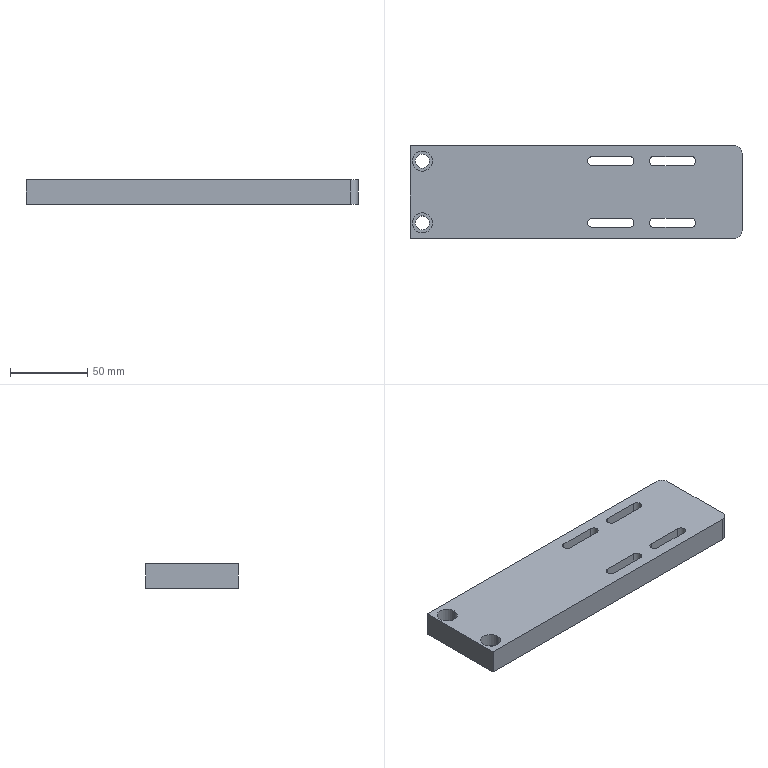CAM job | Mastercam | 3-axis milling, drilling | part box 215 x 60 x 16 mm | stock box 225 x 70 x 20 mm
Tools:
tool_number,name,type,diameter_mm,corner_radius_mm,flutes,flute_length_mm,overall_length_mm,shoulder_length_mm,holder_diameter_mm,length_offset,diameter_offset,default_rpm,default_feed_mm_min,default_plunge_mm_min,coolant
1,5.5 Drill,drill,5.5,0,2,25,50,40,50,1,1,2000,200,600,COOL_OFF
5,5 Flat End Mill,end mill,5,0,4,25,75,25,50,5,5,7000,3000,600,COOL_OFF
6,6 Flat End Mill,end mill,6,0,4,25,75,25,50,6,6,7000,3000,600,COOL_OFF
7,6 Chamfer Mill,chamfer mill,6,0,4,25,75,30,50,7,7,3000,300,600,COOL_OFF
10,10 Flat End Mill,end mill,10,0,4,25,75,25,50,10,10,7000,3500,600,COOL_OFF
21,12 Flat End Mill,end mill,12,0,4,25,75,25,50,21,21,7000,1000,600,COOL_OFF
24,100 Flat End Mill,end mill,100,0,4,25,75,25,50,24,24,4000,1000,600,COOL_OFF
Operations:
seq,operation,operation_type,tool_number,tool_name,tool_diameter_mm,spindle_rpm,feed_mm_min,plunge_mm_min,retract_mm_min,cycle_time_s,wcs,posted,nc_file
1,Facing - [WCS: Plane] - [Tplane: Plane],Facing,24,100 Flat End Mill,100,4000,1000,600,1200,27.035,Plane,yes,.nc
2,2D High Speed (2D Dynamic Mill) - [WCS: Plane] - [Tplane: Plane],HighSpeed2D,10,10 Flat End Mill,10,7000,3000,600,1200,49.134,Plane,yes,.nc
3,Drill/Counterbore - [WCS: Plane] - [Tplane: Plane],Drill,7,6 Chamfer Mill,6,3000,300,600,1200,8.186,Plane,yes,.nc
4,Peck Drill - [WCS: Plane] - [Tplane: Plane],Drill,1,5.5 Drill,5.5,2000,200,600,1200,71.414,Plane,yes,.nc
5,Helix Bore - [WCS: Plane] - [Tplane: Plane],HelixBore,6,6 Flat End Mill,6,7000,3000,600,1200,33.041,Plane,yes,.nc
6,Contour (Ramp) - [WCS: Plane] - [Tplane: Plane],Contour,5,5 Flat End Mill,5,7000,3000,600,1200,73.747,Plane,yes,.nc
7,Helix Bore - [WCS: Plane] - [Tplane: Plane],HelixBore,5,5 Flat End Mill,5,7000,3000,600,1200,18.5,Plane,yes,.nc
8,Contour (Ramp) - [WCS: Plane] - [Tplane: Plane],Contour,5,5 Flat End Mill,5,7000,1500,600,1200,139.774,Plane,yes,.nc
9,Contour (2D) - [WCS: Plane] - [Tplane: Plane],Contour,21,12 Flat End Mill,12,7000,1000,600,1200,35.718,Plane,yes,.nc
10,Model Chamfer - [WCS: Plane] - [Tplane: Plane],ModelChamfer,7,6 Chamfer Mill,6,7000,1000,600,1200,60.439,Plane,yes,.nc
11,Facing - [WCS: Plane-1] - [Tplane: Plane-1],Facing,24,100 Flat End Mill,100,4000,3000,600,1200,98.284,Plane-1,yes,.nc
12,Contour (2D chamfer) - [WCS: Plane-1] - [Tplane: Plane-1],Contour,7,6 Chamfer Mill,6,7000,1000,600,1200,54.745,Plane-1,yes,.nc